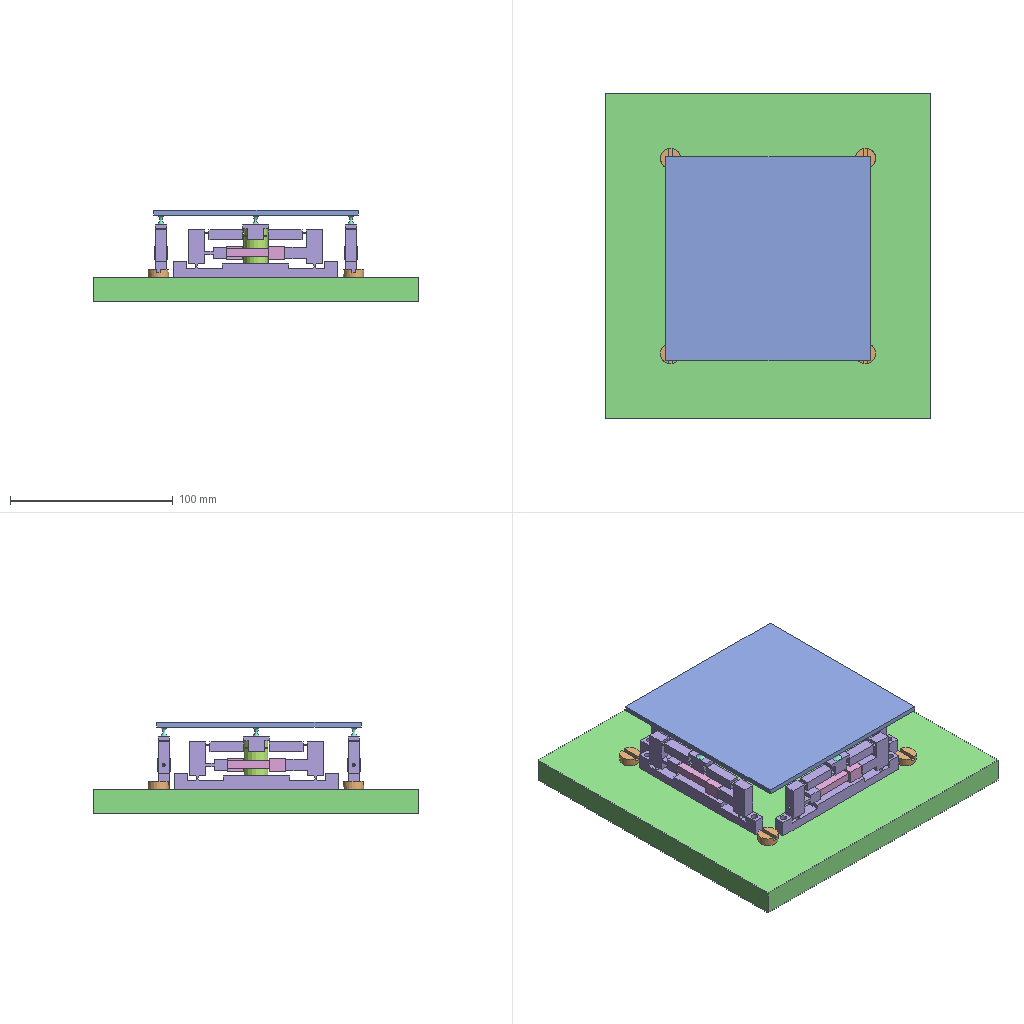Assembly | NX | 10 different items | 22 placed | box 200 x 200 x 56 mm
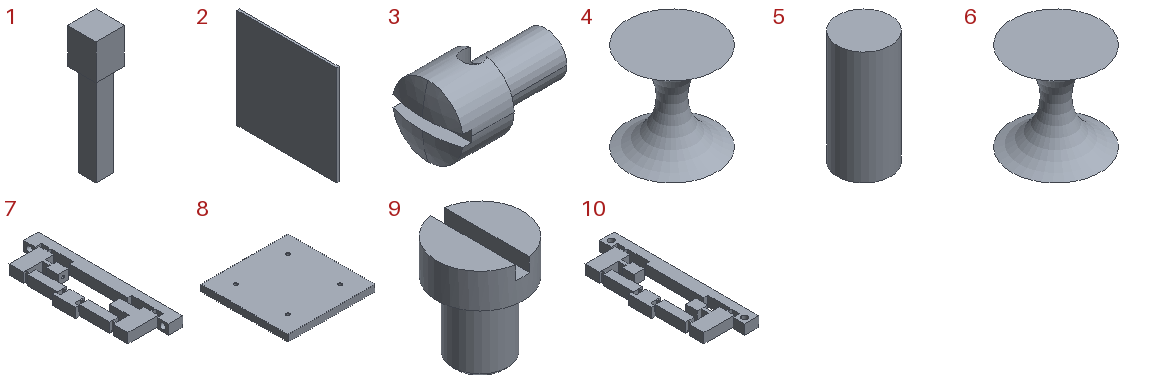Parts list (item | quantity | size | volume | features):
1 | x4 | 8 x 8 x 36 mm | 1290 mm3 | features DATUM_CSYS 3, EXTRUDE 2, SKETCH 2
2 | x1 | 3 x 125.6 x 125.6 mm | 47326 mm3 | features DATUM_CSYS 2, EXTRUDE 1, SKETCH 1
3 | x1 | 8.99 x 5 x 5 mm | 97.359 mm3 | features BREP 1
4 | x1 | 6 x 6 x 6 mm | 40.648 mm3 | features DATUM_CSYS 2, SKETCH 1, SWP104 1
5 | x1 | 15 x 15 x 32.2 mm | 5690 mm3 | features DATUM_CSYS 2, EXTRUDE 1, SKETCH 1
6 | x4 | 6 x 6 x 6 mm | 40.648 mm3 | features DATUM_CSYS 2, SKETCH 1, SWP104 1
7 | x4 | 32.2 x 100.6 x 6.8 mm | 11129 mm3 | features DATUM_CSYS 5, SKETCH 5, EXTRUDE 4, EXTRACT_FACE 2, BREP 1, CHAMFER 1, HOLE PACKAGE 1, Instance Feature 1, Mirror Feature 1, OFFSET_REGION 1, SIMPLE HOLE 1
8 | x1 | 200 x 200 x 15 mm | 597996 mm3 | features DATUM_CSYS 6, EXTRACT_FACE 6, SKETCH 5, HOLE PACKAGE 4, SIMPLE HOLE 4, SYMBOLIC_THREAD 4, Instance Feature 2, Mirror Feature 2, EXTRUDE 1
9 | x4 | 12.5 x 12.5 x 15 mm | 1063 mm3 | features DATUM_CSYS 4, EXTRUDE 3, SKETCH 3, CHAMFER 1
10 | x1 | 32.2 x 100.6 x 6.8 mm | 11071 mm3 | features BREP 1
Mates (type | each side: item.copy, entity, surface, feature):
Fix | 8.1 component
Touch | 7.1 face plane Body(0) | 8.1 face plane Extrude(1) | 2 times
Distance | 7.1 face plane Body(0) | 8.1 face plane Extrude(1) | 3 times
Distance | 7.1 face plane Body(0) | 7.1 face plane Body(0)
Concentric | 9.1 edge | 8.1 edge | 4 times
Touch | 6.1 face plane Revolve(1) | 7.1 face plane Body(0) | 2 times
Touch | 1.1 face plane Extrude(2) | 7.1 face plane Body(0) | 2 times
Distance | 1.1 face plane Extrude(2) | 7.1 face plane Body(0) | 5 times
Distance | 5.1 face cylinder Extrude(1) | 7.1 face plane Body(0) | 2 times
Fix | 7.1 component
Touch | 5.1 face plane Extrude(1) | 8.1 face plane Extrude(1)
Distance | 6.1 face surfaceofrevolution Revolve(1) | 7.1 face plane Body(0)
Distance | 2.1 face plane Extrude(1) | 7.1 face plane Body(0) | 3 times
Concentric | 4.1 edge | 5.1 edge